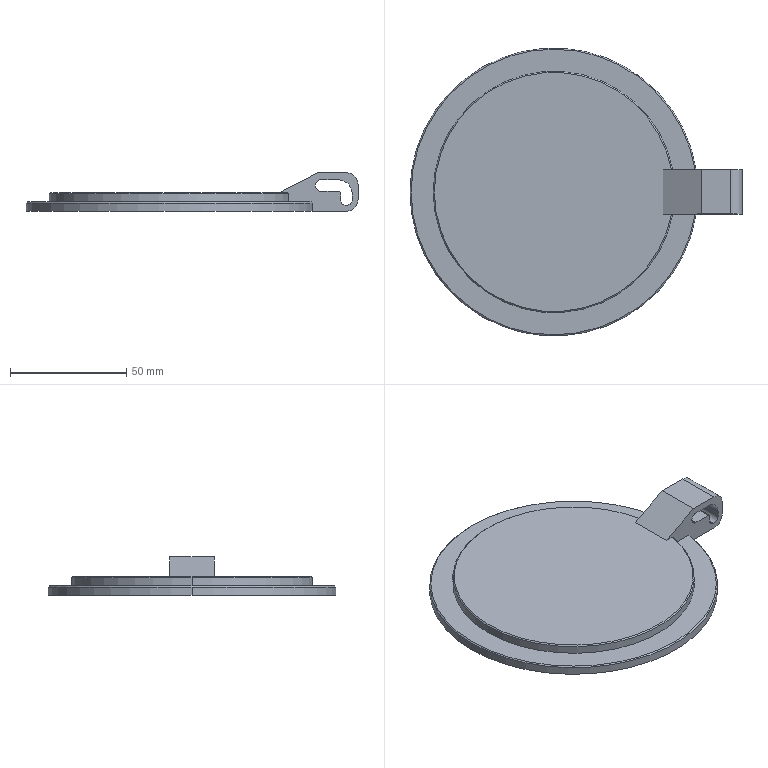Part | SolidWorks | features ICE 2, Chamfer 1, Extrusion 1, Fillet 1 | 1 solid | 27 faces | box 143 x 124 x 16.5 mm | volume 87998 mm3 | plane 12 | cylinder 11 | cone 4 | commonest cylinder face diameters 5 x3 10 x2 104 x2 124 x2 2 x1 12 x1
STEP:
#1=CARTESIAN_POINT('',(-51.5,0.,8.));
#2=VERTEX_POINT('',#1);
#3=CARTESIAN_POINT('',(50.616,-9.5,8.));
#4=VERTEX_POINT('',#3);
#5=CARTESIAN_POINT('',(0.,0.,8.));
#6=DIRECTION('',(0.,0.,1.));
#7=DIRECTION('',(1.,0.,0.));
#8=AXIS2_PLACEMENT_3D('',#5,#6,#7);
#9=CIRCLE('',#8,51.5);
#10=EDGE_CURVE('',#2,#4,#9,.T.);
#11=ORIENTED_EDGE('',*,*,#10,.F.);
#12=CARTESIAN_POINT('',(-52.,0.,7.5));
#13=VERTEX_POINT('',#12);
#14=CARTESIAN_POINT('',(-51.5,0.,8.));
#15=DIRECTION('',(-0.7071,0.,-0.7071));
#16=VECTOR('',#15,1000.);
#17=LINE('',#14,#16);
#18=EDGE_CURVE('',#2,#13,#17,.T.);
#19=ORIENTED_EDGE('',*,*,#18,.T.);
#20=CARTESIAN_POINT('',(51.125,-9.5,7.5));
#21=VERTEX_POINT('',#20);
#22=CARTESIAN_POINT('',(0.,0.,7.5));
#23=DIRECTION('',(0.,0.,-1.));
#24=DIRECTION('',(1.,0.,0.));
#25=AXIS2_PLACEMENT_3D('',#22,#23,#24);
#26=CIRCLE('',#25,52.);
#27=EDGE_CURVE('',#21,#13,#26,.T.);
#28=ORIENTED_EDGE('',*,*,#27,.F.);
#29=CARTESIAN_POINT('',(50.616,-9.5,8.));
#30=CARTESIAN_POINT('',(50.786,-9.5,7.833));
#31=CARTESIAN_POINT('',(50.955,-9.5,7.667));
#32=CARTESIAN_POINT('',(51.125,-9.5,7.5));
#33=B_SPLINE_CURVE_WITH_KNOTS('',3,(#29,#30,#31,#32),.UNSPECIFIED.,.F.,.F.,(4,4),(0.,0.0007132),.UNSPECIFIED.);
#34=EDGE_CURVE('',#4,#21,#33,.T.);
#35=ORIENTED_EDGE('',*,*,#34,.F.);
#36=EDGE_LOOP('',(#11,#19,#28,#35));
#37=FACE_OUTER_BOUND('',#36,.T.);
#38=CARTESIAN_POINT('',(0.,0.,8.));
#39=DIRECTION('',(0.,0.,-1.));
#40=DIRECTION('',(-1.,0.,0.));
#41=AXIS2_PLACEMENT_3D('',#38,#39,#40);
#42=CONICAL_SURFACE('',#41,51.5,0.7854);
#43=ADVANCED_FACE('',(#37),#42,.T.);
#44=CARTESIAN_POINT('',(-61.5,0.,4.));
#45=VERTEX_POINT('',#44);
#46=CARTESIAN_POINT('',(60.762,-9.5,4.));
#47=VERTEX_POINT('',#46);
#48=CARTESIAN_POINT('',(0.,0.,4.));
#49=DIRECTION('',(0.,0.,1.));
#50=DIRECTION('',(1.,0.,0.));
#51=AXIS2_PLACEMENT_3D('',#48,#49,#50);
#52=CIRCLE('',#51,61.5);
#53=EDGE_CURVE('',#45,#47,#52,.T.);
#54=ORIENTED_EDGE('',*,*,#53,.F.);
#55=CARTESIAN_POINT('',(-62.,0.,3.5));
#56=VERTEX_POINT('',#55);
#57=CARTESIAN_POINT('',(-61.5,0.,4.));
#58=DIRECTION('',(-0.7071,0.,-0.7071));
#59=VECTOR('',#58,1000.);
#60=LINE('',#57,#59);
#61=EDGE_CURVE('',#45,#56,#60,.T.);
#62=ORIENTED_EDGE('',*,*,#61,.T.);
#63=CARTESIAN_POINT('',(61.268,-9.5,3.5));
#64=VERTEX_POINT('',#63);
#65=CARTESIAN_POINT('',(0.,0.,3.5));
#66=DIRECTION('',(0.,0.,-1.));
#67=DIRECTION('',(1.,0.,0.));
#68=AXIS2_PLACEMENT_3D('',#65,#66,#67);
#69=CIRCLE('',#68,62.);
#70=EDGE_CURVE('',#64,#56,#69,.T.);
#71=ORIENTED_EDGE('',*,*,#70,.F.);
#72=CARTESIAN_POINT('',(60.762,-9.5,4.));
#73=CARTESIAN_POINT('',(60.931,-9.5,3.833));
#74=CARTESIAN_POINT('',(61.099,-9.5,3.667));
#75=CARTESIAN_POINT('',(61.268,-9.5,3.5));
#76=B_SPLINE_CURVE_WITH_KNOTS('',3,(#72,#73,#74,#75),.UNSPECIFIED.,.F.,.F.,(4,4),(0.,0.0007114),.UNSPECIFIED.);
#77=EDGE_CURVE('',#47,#64,#76,.T.);
#78=ORIENTED_EDGE('',*,*,#77,.F.);
#79=EDGE_LOOP('',(#54,#62,#71,#78));
#80=FACE_OUTER_BOUND('',#79,.T.);
#81=CARTESIAN_POINT('',(0.,0.,4.));
#82=DIRECTION('',(0.,0.,-1.));
#83=DIRECTION('',(-1.,0.,0.));
#84=AXIS2_PLACEMENT_3D('',#81,#82,#83);
#85=CONICAL_SURFACE('',#84,61.5,0.7854);
#86=ADVANCED_FACE('',(#80),#85,.T.);
#87=CARTESIAN_POINT('',(78.5,9.5,5.));
#88=VERTEX_POINT('',#87);
#89=CARTESIAN_POINT('',(76.,9.5,2.5));
#90=VERTEX_POINT('',#89);
#91=CARTESIAN_POINT('',(76.,9.5,5.));
#92=DIRECTION('',(0.,1.,0.));
#93=DIRECTION('',(0.,0.,1.));
#94=AXIS2_PLACEMENT_3D('',#91,#92,#93);
#95=CIRCLE('',#94,2.5);
#96=EDGE_CURVE('',#88,#90,#95,.T.);
#97=ORIENTED_EDGE('',*,*,#96,.T.);
#98=CARTESIAN_POINT('',(76.,-9.5,2.5));
#99=VERTEX_POINT('',#98);
#100=CARTESIAN_POINT('',(76.,9.5,2.5));
#101=DIRECTION('',(0.,-1.,0.));
#102=VECTOR('',#101,1000.);
#103=LINE('',#100,#102);
#104=EDGE_CURVE('',#90,#99,#103,.T.);
#105=ORIENTED_EDGE('',*,*,#104,.T.);
#106=CARTESIAN_POINT('',(78.5,-9.5,5.));
#107=VERTEX_POINT('',#106);
#108=CARTESIAN_POINT('',(76.,-9.5,5.));
#109=DIRECTION('',(0.,1.,0.));
#110=DIRECTION('',(0.,0.,1.));
#111=AXIS2_PLACEMENT_3D('',#108,#109,#110);
#112=CIRCLE('',#111,2.5);
#113=EDGE_CURVE('',#107,#99,#112,.T.);
#114=ORIENTED_EDGE('',*,*,#113,.F.);
#115=CARTESIAN_POINT('',(78.5,9.5,5.));
#116=DIRECTION('',(0.,-1.,0.));
#117=VECTOR('',#116,1000.);
#118=LINE('',#115,#117);
#119=EDGE_CURVE('',#88,#107,#118,.T.);
#120=ORIENTED_EDGE('',*,*,#119,.F.);
#121=EDGE_LOOP('',(#97,#105,#114,#120));
#122=FACE_OUTER_BOUND('',#121,.T.);
#123=CARTESIAN_POINT('',(76.,9.5,5.));
#124=DIRECTION('',(0.,-1.,0.));
#125=DIRECTION('',(0.,0.,-1.));
#126=AXIS2_PLACEMENT_3D('',#123,#124,#125);
#127=CYLINDRICAL_SURFACE('',#126,2.5);
#128=ADVANCED_FACE('',(#122),#127,.F.);
#129=ORIENTED_EDGE('',*,*,#27,.T.);
#130=CARTESIAN_POINT('',(-52.,0.,4.));
#131=VERTEX_POINT('',#130);
#132=CARTESIAN_POINT('',(-52.,0.,8.));
#133=DIRECTION('',(0.,0.,-1.));
#134=VECTOR('',#133,1000.);
#135=LINE('',#132,#134);
#136=EDGE_CURVE('',#13,#131,#135,.T.);
#137=ORIENTED_EDGE('',*,*,#136,.T.);
#138=CARTESIAN_POINT('',(51.125,-9.5,4.));
#139=VERTEX_POINT('',#138);
#140=CARTESIAN_POINT('',(0.,0.,4.));
#141=DIRECTION('',(0.,0.,1.));
#142=DIRECTION('',(1.,0.,0.));
#143=AXIS2_PLACEMENT_3D('',#140,#141,#142);
#144=CIRCLE('',#143,52.);
#145=EDGE_CURVE('',#131,#139,#144,.T.);
#146=ORIENTED_EDGE('',*,*,#145,.T.);
#147=CARTESIAN_POINT('',(51.125,-9.5,8.));
#148=DIRECTION('',(0.,0.,1.));
#149=VECTOR('',#148,1000.);
#150=LINE('',#147,#149);
#151=EDGE_CURVE('',#139,#21,#150,.T.);
#152=ORIENTED_EDGE('',*,*,#151,.T.);
#153=EDGE_LOOP('',(#129,#137,#146,#152));
#154=FACE_OUTER_BOUND('',#153,.T.);
#155=CARTESIAN_POINT('',(0.,0.,8.));
#156=DIRECTION('',(0.,0.,-1.));
#157=DIRECTION('',(-1.,0.,0.));
#158=AXIS2_PLACEMENT_3D('',#155,#156,#157);
#159=CYLINDRICAL_SURFACE('',#158,52.);
#160=ADVANCED_FACE('',(#154),#159,.T.);
#161=ORIENTED_EDGE('',*,*,#70,.T.);
#162=CARTESIAN_POINT('',(-62.,0.,0.));
#163=VERTEX_POINT('',#162);
#164=CARTESIAN_POINT('',(-62.,0.,4.));
#165=DIRECTION('',(0.,0.,-1.));
#166=VECTOR('',#165,1000.);
#167=LINE('',#164,#166);
#168=EDGE_CURVE('',#56,#163,#167,.T.);
#169=ORIENTED_EDGE('',*,*,#168,.T.);
#170=CARTESIAN_POINT('',(61.268,-9.5,0.));
#171=VERTEX_POINT('',#170);
#172=CARTESIAN_POINT('',(0.,0.,0.));
#173=DIRECTION('',(0.,0.,1.));
#174=DIRECTION('',(1.,0.,0.));
#175=AXIS2_PLACEMENT_3D('',#172,#173,#174);
#176=CIRCLE('',#175,62.);
#177=EDGE_CURVE('',#163,#171,#176,.T.);
#178=ORIENTED_EDGE('',*,*,#177,.T.);
#179=CARTESIAN_POINT('',(61.268,-9.5,4.));
#180=DIRECTION('',(0.,0.,1.));
#181=VECTOR('',#180,1000.);
#182=LINE('',#179,#181);
#183=EDGE_CURVE('',#171,#64,#182,.T.);
#184=ORIENTED_EDGE('',*,*,#183,.T.);
#185=EDGE_LOOP('',(#161,#169,#178,#184));
#186=FACE_OUTER_BOUND('',#185,.T.);
#187=CARTESIAN_POINT('',(0.,0.,4.));
#188=DIRECTION('',(0.,0.,-1.));
#189=DIRECTION('',(-1.,0.,0.));
#190=AXIS2_PLACEMENT_3D('',#187,#188,#189);
#191=CYLINDRICAL_SURFACE('',#190,62.);
#192=ADVANCED_FACE('',(#186),#191,.T.);
#193=ORIENTED_EDGE('',*,*,#168,.F.);
#194=CARTESIAN_POINT('',(61.268,9.5,3.5));
#195=VERTEX_POINT('',#194);
#196=CARTESIAN_POINT('',(0.,0.,3.5));
#197=DIRECTION('',(0.,0.,-1.));
#198=DIRECTION('',(1.,0.,0.));
#199=AXIS2_PLACEMENT_3D('',#196,#197,#198);
#200=CIRCLE('',#199,62.);
#201=EDGE_CURVE('',#56,#195,#200,.T.);
#202=ORIENTED_EDGE('',*,*,#201,.T.);
#203=CARTESIAN_POINT('',(61.268,9.5,0.));
#204=VERTEX_POINT('',#203);
#205=CARTESIAN_POINT('',(61.268,9.5,4.));
#206=DIRECTION('',(0.,0.,1.));
#207=VECTOR('',#206,1000.);
#208=LINE('',#205,#207);
#209=EDGE_CURVE('',#204,#195,#208,.T.);
#210=ORIENTED_EDGE('',*,*,#209,.F.);
#211=CARTESIAN_POINT('',(0.,0.,0.));
#212=DIRECTION('',(0.,0.,1.));
#213=DIRECTION('',(1.,0.,0.));
#214=AXIS2_PLACEMENT_3D('',#211,#212,#213);
#215=CIRCLE('',#214,62.);
#216=EDGE_CURVE('',#204,#163,#215,.T.);
#217=ORIENTED_EDGE('',*,*,#216,.T.);
#218=EDGE_LOOP('',(#193,#202,#210,#217));
#219=FACE_OUTER_BOUND('',#218,.T.);
#220=CARTESIAN_POINT('',(0.,0.,4.));
#221=DIRECTION('',(0.,0.,-1.));
#222=DIRECTION('',(-1.,0.,0.));
#223=AXIS2_PLACEMENT_3D('',#220,#221,#222);
#224=CYLINDRICAL_SURFACE('',#223,62.);
#225=ADVANCED_FACE('',(#219),#224,.T.);
#226=CARTESIAN_POINT('',(51.125,9.5,4.));
#227=VERTEX_POINT('',#226);
#228=CARTESIAN_POINT('',(60.762,9.5,4.));
#229=VERTEX_POINT('',#228);
#230=CARTESIAN_POINT('',(0.,9.5,4.));
#231=DIRECTION('',(1.,0.,0.));
#232=VECTOR('',#231,1000.);
#233=LINE('',#230,#232);
#234=EDGE_CURVE('',#227,#229,#233,.T.);
#235=ORIENTED_EDGE('',*,*,#234,.T.);
#236=CARTESIAN_POINT('',(0.,0.,4.));
#237=DIRECTION('',(0.,0.,1.));
#238=DIRECTION('',(1.,0.,0.));
#239=AXIS2_PLACEMENT_3D('',#236,#237,#238);
#240=CIRCLE('',#239,61.5);
#241=EDGE_CURVE('',#229,#45,#240,.T.);
#242=ORIENTED_EDGE('',*,*,#241,.T.);
#243=ORIENTED_EDGE('',*,*,#53,.T.);
#244=CARTESIAN_POINT('',(0.,-9.5,4.));
#245=DIRECTION('',(1.,0.,0.));
#246=VECTOR('',#245,1000.);
#247=LINE('',#244,#246);
#248=EDGE_CURVE('',#139,#47,#247,.T.);
#249=ORIENTED_EDGE('',*,*,#248,.F.);
#250=ORIENTED_EDGE('',*,*,#145,.F.);
#251=CARTESIAN_POINT('',(0.,0.,4.));
#252=DIRECTION('',(0.,0.,1.));
#253=DIRECTION('',(1.,0.,0.));
#254=AXIS2_PLACEMENT_3D('',#251,#252,#253);
#255=CIRCLE('',#254,52.);
#256=EDGE_CURVE('',#227,#131,#255,.T.);
#257=ORIENTED_EDGE('',*,*,#256,.F.);
#258=EDGE_LOOP('',(#235,#242,#243,#249,#250,#257));
#259=FACE_OUTER_BOUND('',#258,.T.);
#260=CARTESIAN_POINT('',(0.,0.,4.));
#261=DIRECTION('',(0.,0.,1.));
#262=DIRECTION('',(1.,0.,0.));
#263=AXIS2_PLACEMENT_3D('',#260,#261,#262);
#264=PLANE('',#263);
#265=ADVANCED_FACE('',(#259),#264,.T.);
#266=ORIENTED_EDGE('',*,*,#136,.F.);
#267=CARTESIAN_POINT('',(51.125,9.5,7.5));
#268=VERTEX_POINT('',#267);
#269=CARTESIAN_POINT('',(0.,0.,7.5));
#270=DIRECTION('',(0.,0.,-1.));
#271=DIRECTION('',(1.,0.,0.));
#272=AXIS2_PLACEMENT_3D('',#269,#270,#271);
#273=CIRCLE('',#272,52.);
#274=EDGE_CURVE('',#13,#268,#273,.T.);
#275=ORIENTED_EDGE('',*,*,#274,.T.);
#276=CARTESIAN_POINT('',(51.125,9.5,8.));
#277=DIRECTION('',(0.,0.,1.));
#278=VECTOR('',#277,1000.);
#279=LINE('',#276,#278);
#280=EDGE_CURVE('',#227,#268,#279,.T.);
#281=ORIENTED_EDGE('',*,*,#280,.F.);
#282=ORIENTED_EDGE('',*,*,#256,.T.);
#283=EDGE_LOOP('',(#266,#275,#281,#282));
#284=FACE_OUTER_BOUND('',#283,.T.);
#285=CARTESIAN_POINT('',(0.,0.,8.));
#286=DIRECTION('',(0.,0.,-1.));
#287=DIRECTION('',(-1.,0.,0.));
#288=AXIS2_PLACEMENT_3D('',#285,#286,#287);
#289=CYLINDRICAL_SURFACE('',#288,52.);
#290=ADVANCED_FACE('',(#284),#289,.T.);
#291=CARTESIAN_POINT('',(47.,9.5,8.));
#292=VERTEX_POINT('',#291);
#293=CARTESIAN_POINT('',(50.616,9.5,8.));
#294=VERTEX_POINT('',#293);
#295=CARTESIAN_POINT('',(0.,9.5,8.));
#296=DIRECTION('',(1.,0.,0.));
#297=VECTOR('',#296,1000.);
#298=LINE('',#295,#297);
#299=EDGE_CURVE('',#292,#294,#298,.T.);
#300=ORIENTED_EDGE('',*,*,#299,.T.);
#301=CARTESIAN_POINT('',(0.,0.,8.));
#302=DIRECTION('',(0.,0.,1.));
#303=DIRECTION('',(1.,0.,0.));
#304=AXIS2_PLACEMENT_3D('',#301,#302,#303);
#305=CIRCLE('',#304,51.5);
#306=EDGE_CURVE('',#294,#2,#305,.T.);
#307=ORIENTED_EDGE('',*,*,#306,.T.);
#308=ORIENTED_EDGE('',*,*,#10,.T.);
#309=CARTESIAN_POINT('',(47.,-9.5,8.));
#310=VERTEX_POINT('',#309);
#311=CARTESIAN_POINT('',(0.,-9.5,8.));
#312=DIRECTION('',(1.,0.,0.));
#313=VECTOR('',#312,1000.);
#314=LINE('',#311,#313);
#315=EDGE_CURVE('',#310,#4,#314,.T.);
#316=ORIENTED_EDGE('',*,*,#315,.F.);
#317=CARTESIAN_POINT('',(47.,9.5,8.));
#318=DIRECTION('',(0.,-1.,0.));
#319=VECTOR('',#318,1000.);
#320=LINE('',#317,#319);
#321=EDGE_CURVE('',#292,#310,#320,.T.);
#322=ORIENTED_EDGE('',*,*,#321,.F.);
#323=EDGE_LOOP('',(#300,#307,#308,#316,#322));
#324=FACE_OUTER_BOUND('',#323,.T.);
#325=CARTESIAN_POINT('',(0.,0.,8.));
#326=DIRECTION('',(0.,0.,1.));
#327=DIRECTION('',(1.,0.,0.));
#328=AXIS2_PLACEMENT_3D('',#325,#326,#327);
#329=PLANE('',#328);
#330=ADVANCED_FACE('',(#324),#329,.T.);
#331=CARTESIAN_POINT('',(76.,9.5,0.));
#332=VERTEX_POINT('',#331);
#333=CARTESIAN_POINT('',(47.,9.5,0.));
#334=DIRECTION('',(-1.,0.,0.));
#335=VECTOR('',#334,1000.);
#336=LINE('',#333,#335);
#337=EDGE_CURVE('',#332,#204,#336,.T.);
#338=ORIENTED_EDGE('',*,*,#337,.F.);
#339=CARTESIAN_POINT('',(76.,-9.5,0.));
#340=VERTEX_POINT('',#339);
#341=CARTESIAN_POINT('',(76.,0.,0.));
#342=DIRECTION('',(0.,-1.,0.));
#343=VECTOR('',#342,1000.);
#344=LINE('',#341,#343);
#345=EDGE_CURVE('',#332,#340,#344,.T.);
#346=ORIENTED_EDGE('',*,*,#345,.T.);
#347=CARTESIAN_POINT('',(47.,-9.5,0.));
#348=DIRECTION('',(-1.,0.,0.));
#349=VECTOR('',#348,1000.);
#350=LINE('',#347,#349);
#351=EDGE_CURVE('',#340,#171,#350,.T.);
#352=ORIENTED_EDGE('',*,*,#351,.T.);
#353=ORIENTED_EDGE('',*,*,#177,.F.);
#354=ORIENTED_EDGE('',*,*,#216,.F.);
#355=EDGE_LOOP('',(#338,#346,#352,#353,#354));
#356=FACE_OUTER_BOUND('',#355,.T.);
#357=CARTESIAN_POINT('',(0.,0.,0.));
#358=DIRECTION('',(0.,0.,1.));
#359=DIRECTION('',(1.,0.,0.));
#360=AXIS2_PLACEMENT_3D('',#357,#358,#359);
#361=PLANE('',#360);
#362=ADVANCED_FACE('',(#356),#361,.F.);
#363=CARTESIAN_POINT('',(65.,9.5,8.5));
#364=VERTEX_POINT('',#363);
#365=CARTESIAN_POINT('',(65.,9.5,13.5));
#366=VERTEX_POINT('',#365);
#367=CARTESIAN_POINT('',(65.,9.5,11.));
#368=DIRECTION('',(0.,1.,0.));
#369=DIRECTION('',(0.,0.,1.));
#370=AXIS2_PLACEMENT_3D('',#367,#368,#369);
#371=CIRCLE('',#370,2.5);
#372=EDGE_CURVE('',#364,#366,#371,.T.);
#373=ORIENTED_EDGE('',*,*,#372,.F.);
#374=CARTESIAN_POINT('',(72.5,9.5,8.5));
#375=VERTEX_POINT('',#374);
#376=CARTESIAN_POINT('',(65.,9.5,8.5));
#377=DIRECTION('',(-1.,0.,0.));
#378=VECTOR('',#377,1000.);
#379=LINE('',#376,#378);
#380=EDGE_CURVE('',#375,#364,#379,.T.);
#381=ORIENTED_EDGE('',*,*,#380,.F.);
#382=CARTESIAN_POINT('',(73.5,9.5,7.5));
#383=VERTEX_POINT('',#382);
#384=CARTESIAN_POINT('',(72.5,9.5,7.5));
#385=DIRECTION('',(0.,-1.,0.));
#386=DIRECTION('',(0.,0.,-1.));
#387=AXIS2_PLACEMENT_3D('',#384,#385,#386);
#388=CIRCLE('',#387,1.);
#389=EDGE_CURVE('',#383,#375,#388,.T.);
#390=ORIENTED_EDGE('',*,*,#389,.F.);
#391=CARTESIAN_POINT('',(73.5,9.5,5.));
#392=VERTEX_POINT('',#391);
#393=CARTESIAN_POINT('',(73.5,9.5,5.));
#394=DIRECTION('',(0.,0.,1.));
#395=VECTOR('',#394,1000.);
#396=LINE('',#393,#395);
#397=EDGE_CURVE('',#392,#383,#396,.T.);
#398=ORIENTED_EDGE('',*,*,#397,.F.);
#399=CARTESIAN_POINT('',(76.,9.5,5.));
#400=DIRECTION('',(0.,1.,0.));
#401=DIRECTION('',(0.,0.,1.));
#402=AXIS2_PLACEMENT_3D('',#399,#400,#401);
#403=CIRCLE('',#402,2.5);
#404=EDGE_CURVE('',#90,#392,#403,.T.);
#405=ORIENTED_EDGE('',*,*,#404,.F.);
#406=ORIENTED_EDGE('',*,*,#96,.F.);
#407=CARTESIAN_POINT('',(78.5,9.5,7.5));
#408=VERTEX_POINT('',#407);
#409=CARTESIAN_POINT('',(78.5,9.5,5.));
#410=DIRECTION('',(0.,0.,-1.));
#411=VECTOR('',#410,1000.);
#412=LINE('',#409,#411);
#413=EDGE_CURVE('',#408,#88,#412,.T.);
#414=ORIENTED_EDGE('',*,*,#413,.F.);
#415=CARTESIAN_POINT('',(72.5,9.5,13.5));
#416=VERTEX_POINT('',#415);
#417=CARTESIAN_POINT('',(72.5,9.5,7.5));
#418=DIRECTION('',(0.,1.,0.));
#419=DIRECTION('',(0.,0.,-1.));
#420=AXIS2_PLACEMENT_3D('',#417,#418,#419);
#421=CIRCLE('',#420,6.);
#422=EDGE_CURVE('',#416,#408,#421,.T.);
#423=ORIENTED_EDGE('',*,*,#422,.F.);
#424=CARTESIAN_POINT('',(65.,9.5,13.5));
#425=DIRECTION('',(1.,0.,0.));
#426=VECTOR('',#425,1000.);
#427=LINE('',#424,#426);
#428=EDGE_CURVE('',#366,#416,#427,.T.);
#429=ORIENTED_EDGE('',*,*,#428,.F.);
#430=EDGE_LOOP('',(#373,#381,#390,#398,#405,#406,#414,#423,#429));
#431=FACE_BOUND('',#430,.T.);
#432=CARTESIAN_POINT('',(81.,9.5,11.5));
#433=VERTEX_POINT('',#432);
#434=CARTESIAN_POINT('',(81.,9.5,5.));
#435=VERTEX_POINT('',#434);
#436=CARTESIAN_POINT('',(81.,9.5,0.));
#437=DIRECTION('',(0.,0.,-1.));
#438=VECTOR('',#437,1000.);
#439=LINE('',#436,#438);
#440=EDGE_CURVE('',#433,#435,#439,.T.);
#441=ORIENTED_EDGE('',*,*,#440,.T.);
#442=CARTESIAN_POINT('',(76.,9.5,5.));
#443=DIRECTION('',(0.,1.,0.));
#444=DIRECTION('',(0.,0.,-1.));
#445=AXIS2_PLACEMENT_3D('',#442,#443,#444);
#446=CIRCLE('',#445,5.);
#447=EDGE_CURVE('',#435,#332,#446,.T.);
#448=ORIENTED_EDGE('',*,*,#447,.T.);
#449=ORIENTED_EDGE('',*,*,#337,.T.);
#450=ORIENTED_EDGE('',*,*,#209,.T.);
#451=CARTESIAN_POINT('',(61.268,9.5,3.5));
#452=CARTESIAN_POINT('',(61.099,9.5,3.667));
#453=CARTESIAN_POINT('',(60.931,9.5,3.833));
#454=CARTESIAN_POINT('',(60.762,9.5,4.));
#455=B_SPLINE_CURVE_WITH_KNOTS('',3,(#451,#452,#453,#454),.UNSPECIFIED.,.F.,.F.,(4,4),(0.,0.0007114),.UNSPECIFIED.);
#456=EDGE_CURVE('',#195,#229,#455,.T.);
#457=ORIENTED_EDGE('',*,*,#456,.T.);
#458=ORIENTED_EDGE('',*,*,#234,.F.);
#459=ORIENTED_EDGE('',*,*,#280,.T.);
#460=CARTESIAN_POINT('',(51.125,9.5,7.5));
#461=CARTESIAN_POINT('',(50.955,9.5,7.667));
#462=CARTESIAN_POINT('',(50.786,9.5,7.833));
#463=CARTESIAN_POINT('',(50.616,9.5,8.));
#464=B_SPLINE_CURVE_WITH_KNOTS('',3,(#460,#461,#462,#463),.UNSPECIFIED.,.F.,.F.,(4,4),(0.,0.0007132),.UNSPECIFIED.);
#465=EDGE_CURVE('',#268,#294,#464,.T.);
#466=ORIENTED_EDGE('',*,*,#465,.T.);
#467=ORIENTED_EDGE('',*,*,#299,.F.);
#468=CARTESIAN_POINT('',(63.5,9.5,16.5));
#469=VERTEX_POINT('',#468);
#470=CARTESIAN_POINT('',(63.5,9.5,16.5));
#471=DIRECTION('',(0.889,0.,0.458));
#472=VECTOR('',#471,1000.);
#473=LINE('',#470,#472);
#474=EDGE_CURVE('',#292,#469,#473,.T.);
#475=ORIENTED_EDGE('',*,*,#474,.T.);
#476=CARTESIAN_POINT('',(76.,9.5,16.5));
#477=VERTEX_POINT('',#476);
#478=CARTESIAN_POINT('',(76.,9.5,16.5));
#479=DIRECTION('',(1.,0.,0.));
#480=VECTOR('',#479,1000.);
#481=LINE('',#478,#480);
#482=EDGE_CURVE('',#469,#477,#481,.T.);
#483=ORIENTED_EDGE('',*,*,#482,.T.);
#484=CARTESIAN_POINT('',(76.,9.5,11.5));
#485=DIRECTION('',(0.,1.,0.));
#486=DIRECTION('',(0.,0.,-1.));
#487=AXIS2_PLACEMENT_3D('',#484,#485,#486);
#488=CIRCLE('',#487,5.);
#489=EDGE_CURVE('',#477,#433,#488,.T.);
#490=ORIENTED_EDGE('',*,*,#489,.T.);
#491=EDGE_LOOP('',(#441,#448,#449,#450,#457,#458,#459,#466,#467,#475,#483,#490));
#492=FACE_OUTER_BOUND('',#491,.T.);
#493=CARTESIAN_POINT('',(76.,9.5,11.5));
#494=DIRECTION('',(0.,-1.,0.));
#495=DIRECTION('',(0.,0.,-1.));
#496=AXIS2_PLACEMENT_3D('',#493,#494,#495);
#497=PLANE('',#496);
#498=ADVANCED_FACE('',(#431,#492),#497,.F.);
#499=CARTESIAN_POINT('',(72.5,-9.5,8.5));
#500=VERTEX_POINT('',#499);
#501=CARTESIAN_POINT('',(65.,-9.5,8.5));
#502=VERTEX_POINT('',#501);
#503=CARTESIAN_POINT('',(65.,-9.5,8.5));
#504=DIRECTION('',(-1.,0.,0.));
#505=VECTOR('',#504,1000.);
#506=LINE('',#503,#505);
#507=EDGE_CURVE('',#500,#502,#506,.T.);
#508=ORIENTED_EDGE('',*,*,#507,.T.);
#509=CARTESIAN_POINT('',(65.,-9.5,13.5));
#510=VERTEX_POINT('',#509);
#511=CARTESIAN_POINT('',(65.,-9.5,11.));
#512=DIRECTION('',(0.,1.,0.));
#513=DIRECTION('',(0.,0.,1.));
#514=AXIS2_PLACEMENT_3D('',#511,#512,#513);
#515=CIRCLE('',#514,2.5);
#516=EDGE_CURVE('',#502,#510,#515,.T.);
#517=ORIENTED_EDGE('',*,*,#516,.T.);
#518=CARTESIAN_POINT('',(72.5,-9.5,13.5));
#519=VERTEX_POINT('',#518);
#520=CARTESIAN_POINT('',(65.,-9.5,13.5));
#521=DIRECTION('',(1.,0.,0.));
#522=VECTOR('',#521,1000.);
#523=LINE('',#520,#522);
#524=EDGE_CURVE('',#510,#519,#523,.T.);
#525=ORIENTED_EDGE('',*,*,#524,.T.);
#526=CARTESIAN_POINT('',(78.5,-9.5,7.5));
#527=VERTEX_POINT('',#526);
#528=CARTESIAN_POINT('',(72.5,-9.5,7.5));
#529=DIRECTION('',(0.,1.,0.));
#530=DIRECTION('',(0.,0.,-1.));
#531=AXIS2_PLACEMENT_3D('',#528,#529,#530);
#532=CIRCLE('',#531,6.);
#533=EDGE_CURVE('',#519,#527,#532,.T.);
#534=ORIENTED_EDGE('',*,*,#533,.T.);
#535=CARTESIAN_POINT('',(78.5,-9.5,5.));
#536=DIRECTION('',(0.,0.,-1.));
#537=VECTOR('',#536,1000.);
#538=LINE('',#535,#537);
#539=EDGE_CURVE('',#527,#107,#538,.T.);
#540=ORIENTED_EDGE('',*,*,#539,.T.);
#541=ORIENTED_EDGE('',*,*,#113,.T.);
#542=CARTESIAN_POINT('',(73.5,-9.5,5.));
#543=VERTEX_POINT('',#542);
#544=CARTESIAN_POINT('',(76.,-9.5,5.));
#545=DIRECTION('',(0.,1.,0.));
#546=DIRECTION('',(0.,0.,1.));
#547=AXIS2_PLACEMENT_3D('',#544,#545,#546);
#548=CIRCLE('',#547,2.5);
#549=EDGE_CURVE('',#99,#543,#548,.T.);
#550=ORIENTED_EDGE('',*,*,#549,.T.);
#551=CARTESIAN_POINT('',(73.5,-9.5,7.5));
#552=VERTEX_POINT('',#551);
#553=CARTESIAN_POINT('',(73.5,-9.5,5.));
#554=DIRECTION('',(0.,0.,1.));
#555=VECTOR('',#554,1000.);
#556=LINE('',#553,#555);
#557=EDGE_CURVE('',#543,#552,#556,.T.);
#558=ORIENTED_EDGE('',*,*,#557,.T.);
#559=CARTESIAN_POINT('',(72.5,-9.5,7.5));
#560=DIRECTION('',(0.,-1.,0.));
#561=DIRECTION('',(0.,0.,-1.));
#562=AXIS2_PLACEMENT_3D('',#559,#560,#561);
#563=CIRCLE('',#562,1.);
#564=EDGE_CURVE('',#552,#500,#563,.T.);
#565=ORIENTED_EDGE('',*,*,#564,.T.);
#566=EDGE_LOOP('',(#508,#517,#525,#534,#540,#541,#550,#558,#565));
#567=FACE_BOUND('',#566,.T.);
#568=ORIENTED_EDGE('',*,*,#351,.F.);
#569=CARTESIAN_POINT('',(81.,-9.5,5.));
#570=VERTEX_POINT('',#569);
#571=CARTESIAN_POINT('',(76.,-9.5,5.));
#572=DIRECTION('',(0.,-1.,0.));
#573=DIRECTION('',(0.,0.,-1.));
#574=AXIS2_PLACEMENT_3D('',#571,#572,#573);
#575=CIRCLE('',#574,5.);
#576=EDGE_CURVE('',#340,#570,#575,.T.);
#577=ORIENTED_EDGE('',*,*,#576,.T.);
#578=CARTESIAN_POINT('',(81.,-9.5,11.5));
#579=VERTEX_POINT('',#578);
#580=CARTESIAN_POINT('',(81.,-9.5,0.));
#581=DIRECTION('',(0.,0.,-1.));
#582=VECTOR('',#581,1000.);
#583=LINE('',#580,#582);
#584=EDGE_CURVE('',#579,#570,#583,.T.);
#585=ORIENTED_EDGE('',*,*,#584,.F.);
#586=CARTESIAN_POINT('',(76.,-9.5,16.5));
#587=VERTEX_POINT('',#586);
#588=CARTESIAN_POINT('',(76.,-9.5,11.5));
#589=DIRECTION('',(0.,1.,0.));
#590=DIRECTION('',(0.,0.,-1.));
#591=AXIS2_PLACEMENT_3D('',#588,#589,#590);
#592=CIRCLE('',#591,5.);
#593=EDGE_CURVE('',#587,#579,#592,.T.);
#594=ORIENTED_EDGE('',*,*,#593,.F.);
#595=CARTESIAN_POINT('',(63.5,-9.5,16.5));
#596=VERTEX_POINT('',#595);
#597=CARTESIAN_POINT('',(76.,-9.5,16.5));
#598=DIRECTION('',(1.,0.,0.));
#599=VECTOR('',#598,1000.);
#600=LINE('',#597,#599);
#601=EDGE_CURVE('',#596,#587,#600,.T.);
#602=ORIENTED_EDGE('',*,*,#601,.F.);
#603=CARTESIAN_POINT('',(63.5,-9.5,16.5));
#604=DIRECTION('',(0.889,0.,0.458));
#605=VECTOR('',#604,1000.);
#606=LINE('',#603,#605);
#607=EDGE_CURVE('',#310,#596,#606,.T.);
#608=ORIENTED_EDGE('',*,*,#607,.F.);
#609=ORIENTED_EDGE('',*,*,#315,.T.);
#610=ORIENTED_EDGE('',*,*,#34,.T.);
#611=ORIENTED_EDGE('',*,*,#151,.F.);
#612=ORIENTED_EDGE('',*,*,#248,.T.);
#613=ORIENTED_EDGE('',*,*,#77,.T.);
#614=ORIENTED_EDGE('',*,*,#183,.F.);
#615=EDGE_LOOP('',(#568,#577,#585,#594,#602,#608,#609,#610,#611,#612,#613,#614));
#616=FACE_OUTER_BOUND('',#615,.T.);
#617=CARTESIAN_POINT('',(76.,-9.5,11.5));
#618=DIRECTION('',(0.,-1.,0.));
#619=DIRECTION('',(0.,0.,-1.));
#620=AXIS2_PLACEMENT_3D('',#617,#618,#619);
#621=PLANE('',#620);
#622=ADVANCED_FACE('',(#567,#616),#621,.T.);
#623=ORIENTED_EDGE('',*,*,#607,.T.);
#624=CARTESIAN_POINT('',(63.5,9.5,16.5));
#625=DIRECTION('',(0.,-1.,0.));
#626=VECTOR('',#625,1000.);
#627=LINE('',#624,#626);
#628=EDGE_CURVE('',#469,#596,#627,.T.);
#629=ORIENTED_EDGE('',*,*,#628,.F.);
#630=ORIENTED_EDGE('',*,*,#474,.F.);
#631=ORIENTED_EDGE('',*,*,#321,.T.);
#632=EDGE_LOOP('',(#623,#629,#630,#631));
#633=FACE_OUTER_BOUND('',#632,.T.);
#634=CARTESIAN_POINT('',(63.5,9.5,16.5));
#635=DIRECTION('',(0.458,0.,-0.889));
#636=DIRECTION('',(-0.889,0.,-0.458));
#637=AXIS2_PLACEMENT_3D('',#634,#635,#636);
#638=PLANE('',#637);
#639=ADVANCED_FACE('',(#633),#638,.F.);
#640=ORIENTED_EDGE('',*,*,#601,.T.);
#641=CARTESIAN_POINT('',(76.,9.5,16.5));
#642=DIRECTION('',(0.,-1.,0.));
#643=VECTOR('',#642,1000.);
#644=LINE('',#641,#643);
#645=EDGE_CURVE('',#477,#587,#644,.T.);
#646=ORIENTED_EDGE('',*,*,#645,.F.);
#647=ORIENTED_EDGE('',*,*,#482,.F.);
#648=ORIENTED_EDGE('',*,*,#628,.T.);
#649=EDGE_LOOP('',(#640,#646,#647,#648));
#650=FACE_OUTER_BOUND('',#649,.T.);
#651=CARTESIAN_POINT('',(76.,9.5,16.5));
#652=DIRECTION('',(0.,0.,-1.));
#653=DIRECTION('',(-1.,0.,0.));
#654=AXIS2_PLACEMENT_3D('',#651,#652,#653);
#655=PLANE('',#654);
#656=ADVANCED_FACE('',(#650),#655,.F.);
#657=ORIENTED_EDGE('',*,*,#593,.T.);
#658=CARTESIAN_POINT('',(81.,9.5,11.5));
#659=DIRECTION('',(0.,-1.,0.));
#660=VECTOR('',#659,1000.);
#661=LINE('',#658,#660);
#662=EDGE_CURVE('',#433,#579,#661,.T.);
#663=ORIENTED_EDGE('',*,*,#662,.F.);
#664=ORIENTED_EDGE('',*,*,#489,.F.);
#665=ORIENTED_EDGE('',*,*,#645,.T.);
#666=EDGE_LOOP('',(#657,#663,#664,#665));
#667=FACE_OUTER_BOUND('',#666,.T.);
#668=CARTESIAN_POINT('',(76.,9.5,11.5));
#669=DIRECTION('',(0.,-1.,0.));
#670=DIRECTION('',(0.,0.,-1.));
#671=AXIS2_PLACEMENT_3D('',#668,#669,#670);
#672=CYLINDRICAL_SURFACE('',#671,5.);
#673=ADVANCED_FACE('',(#667),#672,.T.);
#674=ORIENTED_EDGE('',*,*,#584,.T.);
#675=CARTESIAN_POINT('',(81.,9.5,5.));
#676=DIRECTION('',(0.,1.,0.));
#677=VECTOR('',#676,1000.);
#678=LINE('',#675,#677);
#679=EDGE_CURVE('',#570,#435,#678,.T.);
#680=ORIENTED_EDGE('',*,*,#679,.T.);
#681=ORIENTED_EDGE('',*,*,#440,.F.);
#682=ORIENTED_EDGE('',*,*,#662,.T.);
#683=EDGE_LOOP('',(#674,#680,#681,#682));
#684=FACE_OUTER_BOUND('',#683,.T.);
#685=CARTESIAN_POINT('',(81.,9.5,0.));
#686=DIRECTION('',(-1.,0.,0.));
#687=DIRECTION('',(0.,0.,1.));
#688=AXIS2_PLACEMENT_3D('',#685,#686,#687);
#689=PLANE('',#688);
#690=ADVANCED_FACE('',(#684),#689,.F.);
#691=ORIENTED_EDGE('',*,*,#516,.F.);
#692=CARTESIAN_POINT('',(65.,9.5,8.5));
#693=DIRECTION('',(0.,-1.,0.));
#694=VECTOR('',#693,1000.);
#695=LINE('',#692,#694);
#696=EDGE_CURVE('',#364,#502,#695,.T.);
#697=ORIENTED_EDGE('',*,*,#696,.F.);
#698=ORIENTED_EDGE('',*,*,#372,.T.);
#699=CARTESIAN_POINT('',(65.,9.5,13.5));
#700=DIRECTION('',(0.,-1.,0.));
#701=VECTOR('',#700,1000.);
#702=LINE('',#699,#701);
#703=EDGE_CURVE('',#366,#510,#702,.T.);
#704=ORIENTED_EDGE('',*,*,#703,.T.);
#705=EDGE_LOOP('',(#691,#697,#698,#704));
#706=FACE_OUTER_BOUND('',#705,.T.);
#707=CARTESIAN_POINT('',(65.,9.5,11.));
#708=DIRECTION('',(0.,-1.,0.));
#709=DIRECTION('',(0.,0.,-1.));
#710=AXIS2_PLACEMENT_3D('',#707,#708,#709);
#711=CYLINDRICAL_SURFACE('',#710,2.5);
#712=ADVANCED_FACE('',(#706),#711,.F.);
#713=ORIENTED_EDGE('',*,*,#524,.F.);
#714=ORIENTED_EDGE('',*,*,#703,.F.);
#715=ORIENTED_EDGE('',*,*,#428,.T.);
#716=CARTESIAN_POINT('',(72.5,9.5,13.5));
#717=DIRECTION('',(0.,-1.,0.));
#718=VECTOR('',#717,1000.);
#719=LINE('',#716,#718);
#720=EDGE_CURVE('',#416,#519,#719,.T.);
#721=ORIENTED_EDGE('',*,*,#720,.T.);
#722=EDGE_LOOP('',(#713,#714,#715,#721));
#723=FACE_OUTER_BOUND('',#722,.T.);
#724=CARTESIAN_POINT('',(65.,9.5,13.5));
#725=DIRECTION('',(0.,0.,-1.));
#726=DIRECTION('',(-1.,0.,0.));
#727=AXIS2_PLACEMENT_3D('',#724,#725,#726);
#728=PLANE('',#727);
#729=ADVANCED_FACE('',(#723),#728,.T.);
#730=ORIENTED_EDGE('',*,*,#533,.F.);
#731=ORIENTED_EDGE('',*,*,#720,.F.);
#732=ORIENTED_EDGE('',*,*,#422,.T.);
#733=CARTESIAN_POINT('',(78.5,9.5,7.5));
#734=DIRECTION('',(0.,-1.,0.));
#735=VECTOR('',#734,1000.);
#736=LINE('',#733,#735);
#737=EDGE_CURVE('',#408,#527,#736,.T.);
#738=ORIENTED_EDGE('',*,*,#737,.T.);
#739=EDGE_LOOP('',(#730,#731,#732,#738));
#740=FACE_OUTER_BOUND('',#739,.T.);
#741=CARTESIAN_POINT('',(72.5,9.5,7.5));
#742=DIRECTION('',(0.,-1.,0.));
#743=DIRECTION('',(0.,0.,-1.));
#744=AXIS2_PLACEMENT_3D('',#741,#742,#743);
#745=CYLINDRICAL_SURFACE('',#744,6.);
#746=ADVANCED_FACE('',(#740),#745,.F.);
#747=ORIENTED_EDGE('',*,*,#539,.F.);
#748=ORIENTED_EDGE('',*,*,#737,.F.);
#749=ORIENTED_EDGE('',*,*,#413,.T.);
#750=ORIENTED_EDGE('',*,*,#119,.T.);
#751=EDGE_LOOP('',(#747,#748,#749,#750));
#752=FACE_OUTER_BOUND('',#751,.T.);
#753=CARTESIAN_POINT('',(78.5,9.5,5.));
#754=DIRECTION('',(-1.,0.,0.));
#755=DIRECTION('',(0.,0.,1.));
#756=AXIS2_PLACEMENT_3D('',#753,#754,#755);
#757=PLANE('',#756);
#758=ADVANCED_FACE('',(#752),#757,.T.);
#759=ORIENTED_EDGE('',*,*,#104,.F.);
#760=ORIENTED_EDGE('',*,*,#404,.T.);
#761=CARTESIAN_POINT('',(73.5,9.5,5.));
#762=DIRECTION('',(0.,-1.,0.));
#763=VECTOR('',#762,1000.);
#764=LINE('',#761,#763);
#765=EDGE_CURVE('',#392,#543,#764,.T.);
#766=ORIENTED_EDGE('',*,*,#765,.T.);
#767=ORIENTED_EDGE('',*,*,#549,.F.);
#768=EDGE_LOOP('',(#759,#760,#766,#767));
#769=FACE_OUTER_BOUND('',#768,.T.);
#770=CARTESIAN_POINT('',(76.,9.5,5.));
#771=DIRECTION('',(0.,-1.,0.));
#772=DIRECTION('',(0.,0.,-1.));
#773=AXIS2_PLACEMENT_3D('',#770,#771,#772);
#774=CYLINDRICAL_SURFACE('',#773,2.5);
#775=ADVANCED_FACE('',(#769),#774,.F.);
#776=ORIENTED_EDGE('',*,*,#557,.F.);
#777=ORIENTED_EDGE('',*,*,#765,.F.);
#778=ORIENTED_EDGE('',*,*,#397,.T.);
#779=CARTESIAN_POINT('',(73.5,9.5,7.5));
#780=DIRECTION('',(0.,-1.,0.));
#781=VECTOR('',#780,1000.);
#782=LINE('',#779,#781);
#783=EDGE_CURVE('',#383,#552,#782,.T.);
#784=ORIENTED_EDGE('',*,*,#783,.T.);
#785=EDGE_LOOP('',(#776,#777,#778,#784));
#786=FACE_OUTER_BOUND('',#785,.T.);
#787=CARTESIAN_POINT('',(73.5,9.5,5.));
#788=DIRECTION('',(1.,0.,0.));
#789=DIRECTION('',(0.,0.,-1.));
#790=AXIS2_PLACEMENT_3D('',#787,#788,#789);
#791=PLANE('',#790);
#792=ADVANCED_FACE('',(#786),#791,.T.);
#793=ORIENTED_EDGE('',*,*,#564,.F.);
#794=ORIENTED_EDGE('',*,*,#783,.F.);
#795=ORIENTED_EDGE('',*,*,#389,.T.);
#796=CARTESIAN_POINT('',(72.5,9.5,8.5));
#797=DIRECTION('',(0.,-1.,0.));
#798=VECTOR('',#797,1000.);
#799=LINE('',#796,#798);
#800=EDGE_CURVE('',#375,#500,#799,.T.);
#801=ORIENTED_EDGE('',*,*,#800,.T.);
#802=EDGE_LOOP('',(#793,#794,#795,#801));
#803=FACE_OUTER_BOUND('',#802,.T.);
#804=CARTESIAN_POINT('',(72.5,9.5,7.5));
#805=DIRECTION('',(0.,-1.,0.));
#806=DIRECTION('',(0.,0.,-1.));
#807=AXIS2_PLACEMENT_3D('',#804,#805,#806);
#808=CYLINDRICAL_SURFACE('',#807,1.);
#809=ADVANCED_FACE('',(#803),#808,.T.);
#810=ORIENTED_EDGE('',*,*,#507,.F.);
#811=ORIENTED_EDGE('',*,*,#800,.F.);
#812=ORIENTED_EDGE('',*,*,#380,.T.);
#813=ORIENTED_EDGE('',*,*,#696,.T.);
#814=EDGE_LOOP('',(#810,#811,#812,#813));
#815=FACE_OUTER_BOUND('',#814,.T.);
#816=CARTESIAN_POINT('',(65.,9.5,8.5));
#817=DIRECTION('',(0.,0.,1.));
#818=DIRECTION('',(1.,0.,0.));
#819=AXIS2_PLACEMENT_3D('',#816,#817,#818);
#820=PLANE('',#819);
#821=ADVANCED_FACE('',(#815),#820,.T.);
#822=ORIENTED_EDGE('',*,*,#447,.F.);
#823=ORIENTED_EDGE('',*,*,#679,.F.);
#824=ORIENTED_EDGE('',*,*,#576,.F.);
#825=ORIENTED_EDGE('',*,*,#345,.F.);
#826=EDGE_LOOP('',(#822,#823,#824,#825));
#827=FACE_OUTER_BOUND('',#826,.T.);
#828=CARTESIAN_POINT('',(76.,0.,5.));
#829=DIRECTION('',(0.,-1.,0.));
#830=DIRECTION('',(0.,0.,-1.));
#831=AXIS2_PLACEMENT_3D('',#828,#829,#830);
#832=CYLINDRICAL_SURFACE('',#831,5.);
#833=ADVANCED_FACE('',(#827),#832,.T.);
#834=ORIENTED_EDGE('',*,*,#61,.F.);
#835=ORIENTED_EDGE('',*,*,#241,.F.);
#836=ORIENTED_EDGE('',*,*,#456,.F.);
#837=ORIENTED_EDGE('',*,*,#201,.F.);
#838=EDGE_LOOP('',(#834,#835,#836,#837));
#839=FACE_OUTER_BOUND('',#838,.T.);
#840=CARTESIAN_POINT('',(0.,0.,4.));
#841=DIRECTION('',(0.,0.,-1.));
#842=DIRECTION('',(-1.,0.,0.));
#843=AXIS2_PLACEMENT_3D('',#840,#841,#842);
#844=CONICAL_SURFACE('',#843,61.5,0.7854);
#845=ADVANCED_FACE('',(#839),#844,.T.);
#846=ORIENTED_EDGE('',*,*,#18,.F.);
#847=ORIENTED_EDGE('',*,*,#306,.F.);
#848=ORIENTED_EDGE('',*,*,#465,.F.);
#849=ORIENTED_EDGE('',*,*,#274,.F.);
#850=EDGE_LOOP('',(#846,#847,#848,#849));
#851=FACE_OUTER_BOUND('',#850,.T.);
#852=CARTESIAN_POINT('',(0.,0.,8.));
#853=DIRECTION('',(0.,0.,-1.));
#854=DIRECTION('',(-1.,0.,0.));
#855=AXIS2_PLACEMENT_3D('',#852,#853,#854);
#856=CONICAL_SURFACE('',#855,51.5,0.7854);
#857=ADVANCED_FACE('',(#851),#856,.T.);
#858=CLOSED_SHELL('',(#43,#86,#128,#160,#192,#225,#265,#290,#330,#362,#498,#622,#639,#656,#673,#690,#712,#729,#746,#758,#775,#792,#809,#821,#833,#845,#857));
#859=MANIFOLD_SOLID_BREP('',#858);
#860=CARTESIAN_POINT('',(0.,0.,0.));
#861=DIRECTION('',(0.,0.,1.));
#862=DIRECTION('',(1.,0.,0.));
#863=AXIS2_PLACEMENT_3D('',#860,#861,#862);
#864=(LENGTH_UNIT()NAMED_UNIT(*)SI_UNIT(.MILLI.,.METRE.));
#865=UNCERTAINTY_MEASURE_WITH_UNIT(LENGTH_MEASURE(0.00001),#864,'','');
#866=(NAMED_UNIT(*)PLANE_ANGLE_UNIT()SI_UNIT($,.RADIAN.));
#867=(NAMED_UNIT(*)SI_UNIT($,.STERADIAN.)SOLID_ANGLE_UNIT());
#868=(GEOMETRIC_REPRESENTATION_CONTEXT(3)GLOBAL_UNCERTAINTY_ASSIGNED_CONTEXT((#865))GLOBAL_UNIT_ASSIGNED_CONTEXT((#864,#866,#867))REPRESENTATION_CONTEXT('',''));
#869=ADVANCED_BREP_SHAPE_REPRESENTATION('',(#859,#863),#868);